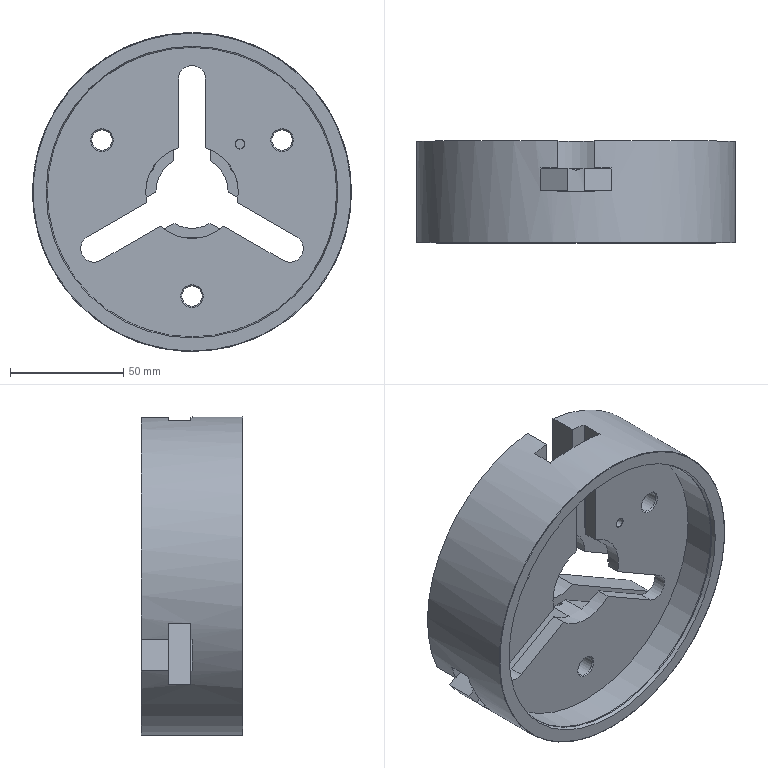Part | 1 solid | 83 faces | box 141 x 45 x 141 mm | volume 361896 mm3 | plane 45 | cylinder 22 | cone 15 | torus 1 | commonest cylinder face diameters 4.2 x3 9 x3 12 x3 14 x3 32 x3 41 x3